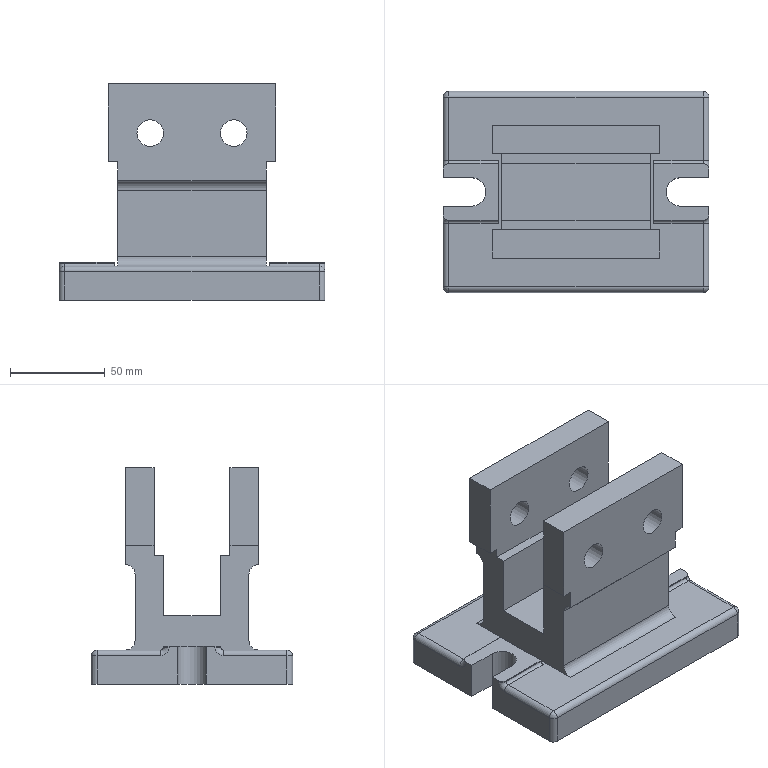Part | NX | features EXTRUDE 8, FACE_BLEND 6, DATUM_CSYS 5, SKETCH 4, BLEND 1 | 1 solid | 79 faces | box 140 x 106 x 114 mm | volume 532545 mm3 | plane 43 | cylinder 28 | torus 4 | sphere 4 | commonest cylinder face diameters 6 x14 3 x4 10 x4 14 x4 15 x2